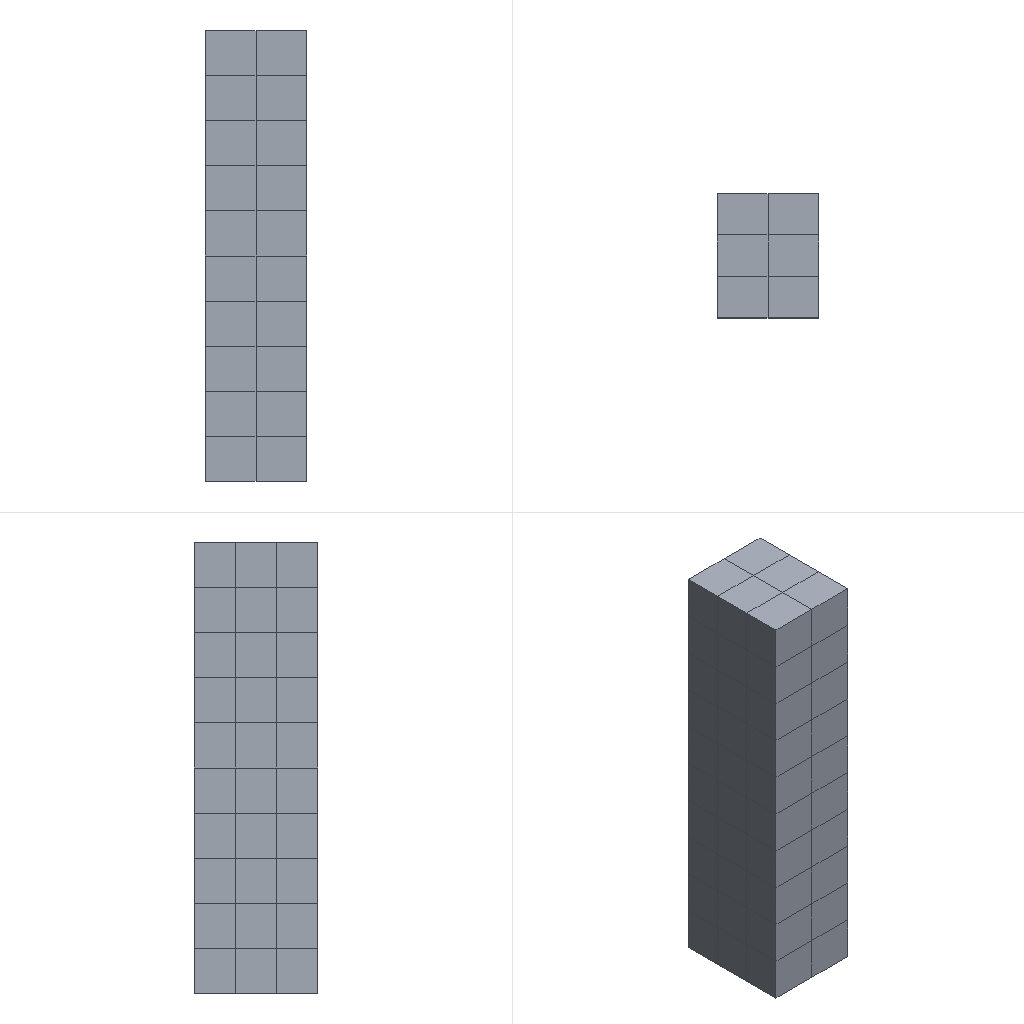Simulation study | abaqus
Set-up summary:
category,name,step,type,value,unit,region
solver,abaqus,,Abaqus/CAE 2024
units,unstated,,unstated
analysis,Step-1,,static,time_period=1
mesh,nodes,,,132
mesh,elements,,,60
element_type,C3D8,,,60
material,Material-1,,behaviors,depvar; user material
section,Material-1,,solid section,,,_PickedSet2
load,Load-1,Step-1,pressure,1e+06,,_PickedSurf5
bc,BC-1,Step-1,fixed,"[dofs=x,y,z n=3]",,_PickedSet4
Abaqus input file, long lists of numbers shortened:
*Heading
** Job name: deck Model name: Model-1
** Generated by: Abaqus/CAE 2024
*Preprint, echo=NO, model=NO, history=NO, contact=NO
**
** PARTS
**
*Part, name=Part-1
*Node
      1,        -8.75,         -15.,         100.
      2,        -8.75,  -5.833,         100.
** (130 more lines like these left out)
*Element, type=C3D8
 1,  45,  46,  50,  49,   1,   2,   6,   5
 2,  46,  47,  51,  50,   2,   3,   7,   6
** (58 more lines like these left out)
*Nset, nset=_PickedSet2, internal, generate
   1,  132,    1
*Elset, elset=_PickedSet2, internal, generate
  1,  60,   1
** Section: Section-1
*Solid Section, elset=_PickedSet2, material=Material-1
,
*End Part
**
**
** ASSEMBLY
**
*Assembly, name=Assembly
**
*Instance, name=Part-1-1, part=Part-1
*End Instance
**
*Nset, nset=_PickedSet4, internal, instance=Part-1-1
  1,  2,  3,  4, 45, 46, 47, 48, 89, 90, 91, 92
*Elset, elset=_PickedSet4, internal, instance=Part-1-1
  1,  2,  3, 31, 32, 33
*Elset, elset=__PickedSurf5_S5, internal, instance=Part-1-1
 28, 29, 30, 58, 59, 60
*Surface, type=ELEMENT, name=_PickedSurf5, internal
__PickedSurf5_S5, S5
*End Assembly
**
** MATERIALS
**
*Material, name=Material-1
*Depvar
      1,
*User Material, constants=2
206000., 0.3
** ----------------------------------------------------------------
**
** STEP: Step-1
**
*Step, name=Step-1, nlgeom=NO
*Static
1., 1., 1e-05, 1.
**
** BOUNDARY CONDITIONS
**
** Name: BC-1 Type: Displacement/Rotation
*Boundary
_PickedSet4, 1, 1
_PickedSet4, 2, 2
_PickedSet4, 3, 3
**
** LOADS
**
** Name: Load-1   Type: Pressure
*Dsload
_PickedSurf5, P, 1e+06
**
** OUTPUT REQUESTS
**
*Restart, write, frequency=0
*Print, solve=NO
**
** FIELD OUTPUT: F-Output-1
**
*Output, field, variable=PRESELECT
**
** HISTORY OUTPUT: H-Output-1
**
*Output, history, variable=PRESELECT
*End Step
Results summary:
result,odb.job_status,,,JOB_STATUS_COMPLETED_SUCCESSFULLY,"consistent, unstated (Abaqus has no unit system)"
result,steps[0].procedure,Step-1,,*STATIC,"consistent, unstated (Abaqus has no unit system)"
result,steps[0].time_period,Step-1,,1,"consistent, unstated (Abaqus has no unit system)"
result,steps[0].n_frames,Step-1,,2,"consistent, unstated (Abaqus has no unit system)"
result,steps[0].last_frame.id,Step-1,,1,"consistent, unstated (Abaqus has no unit system)"
result,steps[0].last_frame.value,Step-1,,1,"consistent, unstated (Abaqus has no unit system)"
result,steps[0].last_frame.description,Step-1,,Increment      1: Step Time =    1.000,"consistent, unstated (Abaqus has no unit system)"
result,steps[0].completed,Step-1,,True,"consistent, unstated (Abaqus has no unit system)"
result,steps[0].max_U_magnitude,Step-1,,481.61,"consistent, unstated (Abaqus has no unit system)"
result,steps[0].max_S_mises,Step-1,,1.08286e+06,"consistent, unstated (Abaqus has no unit system)"
result,steps[0].RF_sum[1],Step-1,,-0.5,"consistent, unstated (Abaqus has no unit system)"
result,steps[0].RF_sum[2],Step-1,,0,"consistent, unstated (Abaqus has no unit system)"
result,steps[0].RF_sum[3],Step-1,,-6.1875e+08,"consistent, unstated (Abaqus has no unit system)"
result,steps[0].diagnostic.n_increments,Step-1,,1,"consistent, unstated (Abaqus has no unit system)"